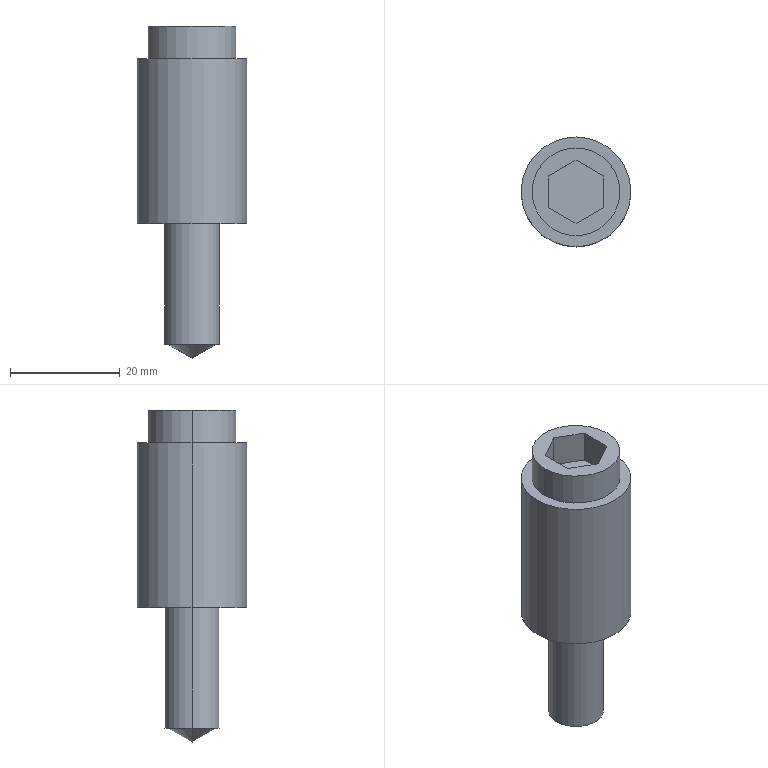Part | Creo | 1 solid | 19 faces | box 20 x 20 x 60.51 mm | volume 11893 mm3 | plane 11 | cylinder 6 | cone 2 | commonest cylinder face diameters 10 x2 16 x2 20 x2
STEP:
#1=CARTESIAN_POINT('',(-211.,254.,30.5));
#2=VERTEX_POINT('',#1);
#3=CARTESIAN_POINT('',(-195.,254.,30.5));
#4=VERTEX_POINT('',#3);
#5=CARTESIAN_POINT('',(-203.,254.,30.5));
#6=DIRECTION('',(0.,0.,1.));
#7=DIRECTION('',(-1.,0.,0.));
#8=AXIS2_PLACEMENT_3D('',#5,#6,#7);
#9=CIRCLE('',#8,8.);
#10=EDGE_CURVE('',#2,#4,#9,.T.);
#11=ORIENTED_EDGE('',*,*,#10,.F.);
#12=CARTESIAN_POINT('',(-203.,254.,30.5));
#13=DIRECTION('',(0.,0.,1.));
#14=DIRECTION('',(1.,0.,0.));
#15=AXIS2_PLACEMENT_3D('',#12,#13,#14);
#16=CIRCLE('',#15,8.);
#17=EDGE_CURVE('',#4,#2,#16,.T.);
#18=ORIENTED_EDGE('',*,*,#17,.F.);
#19=EDGE_LOOP('',(#11,#18));
#20=FACE_OUTER_BOUND('',#19,.F.);
#21=CARTESIAN_POINT('',(-198.,251.113,30.5));
#22=VERTEX_POINT('',#21);
#23=CARTESIAN_POINT('',(-203.,248.226,30.5));
#24=VERTEX_POINT('',#23);
#25=CARTESIAN_POINT('',(-198.,251.113,30.5));
#26=DIRECTION('',(-0.866,-0.5,0.));
#27=VECTOR('',#26,5.774);
#28=LINE('',#25,#27);
#29=EDGE_CURVE('',#22,#24,#28,.T.);
#30=ORIENTED_EDGE('',*,*,#29,.F.);
#31=CARTESIAN_POINT('',(-198.,256.887,30.5));
#32=VERTEX_POINT('',#31);
#33=CARTESIAN_POINT('',(-198.,251.113,30.5));
#34=DIRECTION('',(0.,1.,0.));
#35=VECTOR('',#34,5.774);
#36=LINE('',#33,#35);
#37=EDGE_CURVE('',#22,#32,#36,.T.);
#38=ORIENTED_EDGE('',*,*,#37,.T.);
#39=CARTESIAN_POINT('',(-203.,259.774,30.5));
#40=VERTEX_POINT('',#39);
#41=CARTESIAN_POINT('',(-203.,259.774,30.5));
#42=DIRECTION('',(0.866,-0.5,0.));
#43=VECTOR('',#42,5.774);
#44=LINE('',#41,#43);
#45=EDGE_CURVE('',#40,#32,#44,.T.);
#46=ORIENTED_EDGE('',*,*,#45,.F.);
#47=CARTESIAN_POINT('',(-208.,256.887,30.5));
#48=VERTEX_POINT('',#47);
#49=CARTESIAN_POINT('',(-208.,256.887,30.5));
#50=DIRECTION('',(0.866,0.5,0.));
#51=VECTOR('',#50,5.774);
#52=LINE('',#49,#51);
#53=EDGE_CURVE('',#48,#40,#52,.T.);
#54=ORIENTED_EDGE('',*,*,#53,.F.);
#55=CARTESIAN_POINT('',(-208.,251.113,30.5));
#56=VERTEX_POINT('',#55);
#57=CARTESIAN_POINT('',(-208.,256.887,30.5));
#58=DIRECTION('',(0.,-1.,0.));
#59=VECTOR('',#58,5.774);
#60=LINE('',#57,#59);
#61=EDGE_CURVE('',#48,#56,#60,.T.);
#62=ORIENTED_EDGE('',*,*,#61,.T.);
#63=CARTESIAN_POINT('',(-203.,248.226,30.5));
#64=DIRECTION('',(-0.866,0.5,0.));
#65=VECTOR('',#64,5.774);
#66=LINE('',#63,#65);
#67=EDGE_CURVE('',#24,#56,#66,.T.);
#68=ORIENTED_EDGE('',*,*,#67,.F.);
#69=EDGE_LOOP('',(#30,#38,#46,#54,#62,#68));
#70=FACE_BOUND('',#69,.F.);
#71=CARTESIAN_POINT('',(-203.,254.,30.5));
#72=DIRECTION('',(0.,0.,1.));
#73=DIRECTION('',(1.,0.,0.));
#74=AXIS2_PLACEMENT_3D('',#71,#72,#73);
#75=PLANE('',#74);
#76=ADVANCED_FACE('',(#20,#70),#75,.T.);
#77=CARTESIAN_POINT('',(-195.,254.,24.5));
#78=VERTEX_POINT('',#77);
#79=CARTESIAN_POINT('',(-211.,254.,24.5));
#80=VERTEX_POINT('',#79);
#81=CARTESIAN_POINT('',(-203.,254.,24.5));
#82=DIRECTION('',(0.,0.,-1.));
#83=DIRECTION('',(1.,0.,0.));
#84=AXIS2_PLACEMENT_3D('',#81,#82,#83);
#85=CIRCLE('',#84,8.);
#86=EDGE_CURVE('',#78,#80,#85,.T.);
#87=ORIENTED_EDGE('',*,*,#86,.T.);
#88=CARTESIAN_POINT('',(-211.,254.,24.5));
#89=DIRECTION('',(0.,0.,1.));
#90=VECTOR('',#89,6.);
#91=LINE('',#88,#90);
#92=EDGE_CURVE('',#80,#2,#91,.T.);
#93=ORIENTED_EDGE('',*,*,#92,.T.);
#94=ORIENTED_EDGE('',*,*,#10,.T.);
#95=CARTESIAN_POINT('',(-195.,254.,24.5));
#96=DIRECTION('',(0.,0.,1.));
#97=VECTOR('',#96,6.);
#98=LINE('',#95,#97);
#99=EDGE_CURVE('',#78,#4,#98,.T.);
#100=ORIENTED_EDGE('',*,*,#99,.F.);
#101=EDGE_LOOP('',(#87,#93,#94,#100));
#102=FACE_OUTER_BOUND('',#101,.F.);
#103=CARTESIAN_POINT('',(-203.,254.,-5.5));
#104=DIRECTION('',(0.,0.,1.));
#105=DIRECTION('',(1.,0.,0.));
#106=AXIS2_PLACEMENT_3D('',#103,#104,#105);
#107=CYLINDRICAL_SURFACE('',#106,8.);
#108=ADVANCED_FACE('',(#102),#107,.T.);
#109=CARTESIAN_POINT('',(-213.,254.,24.5));
#110=VERTEX_POINT('',#109);
#111=CARTESIAN_POINT('',(-193.,254.,24.5));
#112=VERTEX_POINT('',#111);
#113=CARTESIAN_POINT('',(-203.,254.,24.5));
#114=DIRECTION('',(0.,0.,1.));
#115=DIRECTION('',(-1.,0.,0.));
#116=AXIS2_PLACEMENT_3D('',#113,#114,#115);
#117=CIRCLE('',#116,10.);
#118=EDGE_CURVE('',#110,#112,#117,.T.);
#119=ORIENTED_EDGE('',*,*,#118,.F.);
#120=CARTESIAN_POINT('',(-203.,254.,24.5));
#121=DIRECTION('',(0.,0.,1.));
#122=DIRECTION('',(1.,0.,0.));
#123=AXIS2_PLACEMENT_3D('',#120,#121,#122);
#124=CIRCLE('',#123,10.);
#125=EDGE_CURVE('',#112,#110,#124,.T.);
#126=ORIENTED_EDGE('',*,*,#125,.F.);
#127=EDGE_LOOP('',(#119,#126));
#128=FACE_OUTER_BOUND('',#127,.F.);
#129=ORIENTED_EDGE('',*,*,#86,.F.);
#130=CARTESIAN_POINT('',(-203.,254.,24.5));
#131=DIRECTION('',(0.,0.,-1.));
#132=DIRECTION('',(-1.,0.,0.));
#133=AXIS2_PLACEMENT_3D('',#130,#131,#132);
#134=CIRCLE('',#133,8.);
#135=EDGE_CURVE('',#80,#78,#134,.T.);
#136=ORIENTED_EDGE('',*,*,#135,.F.);
#137=EDGE_LOOP('',(#129,#136));
#138=FACE_BOUND('',#137,.F.);
#139=CARTESIAN_POINT('',(-203.,254.,24.5));
#140=DIRECTION('',(0.,0.,1.));
#141=DIRECTION('',(1.,0.,0.));
#142=AXIS2_PLACEMENT_3D('',#139,#140,#141);
#143=PLANE('',#142);
#144=ADVANCED_FACE('',(#128,#138),#143,.T.);
#145=ORIENTED_EDGE('',*,*,#135,.T.);
#146=ORIENTED_EDGE('',*,*,#99,.T.);
#147=ORIENTED_EDGE('',*,*,#17,.T.);
#148=ORIENTED_EDGE('',*,*,#92,.F.);
#149=EDGE_LOOP('',(#145,#146,#147,#148));
#150=FACE_OUTER_BOUND('',#149,.F.);
#151=CARTESIAN_POINT('',(-203.,254.,-5.5));
#152=DIRECTION('',(0.,0.,1.));
#153=DIRECTION('',(1.,0.,0.));
#154=AXIS2_PLACEMENT_3D('',#151,#152,#153);
#155=CYLINDRICAL_SURFACE('',#154,8.);
#156=ADVANCED_FACE('',(#150),#155,.T.);
#157=ORIENTED_EDGE('',*,*,#118,.T.);
#158=CARTESIAN_POINT('',(-193.,254.,-5.5));
#159=VERTEX_POINT('',#158);
#160=CARTESIAN_POINT('',(-193.,254.,-5.5));
#161=DIRECTION('',(0.,0.,1.));
#162=VECTOR('',#161,30.);
#163=LINE('',#160,#162);
#164=EDGE_CURVE('',#159,#112,#163,.T.);
#165=ORIENTED_EDGE('',*,*,#164,.F.);
#166=CARTESIAN_POINT('',(-213.,254.,-5.5));
#167=VERTEX_POINT('',#166);
#168=CARTESIAN_POINT('',(-203.,254.,-5.5));
#169=DIRECTION('',(0.,0.,-1.));
#170=DIRECTION('',(1.,0.,0.));
#171=AXIS2_PLACEMENT_3D('',#168,#169,#170);
#172=CIRCLE('',#171,10.);
#173=EDGE_CURVE('',#159,#167,#172,.T.);
#174=ORIENTED_EDGE('',*,*,#173,.T.);
#175=CARTESIAN_POINT('',(-213.,254.,-5.5));
#176=DIRECTION('',(0.,0.,1.));
#177=VECTOR('',#176,30.);
#178=LINE('',#175,#177);
#179=EDGE_CURVE('',#167,#110,#178,.T.);
#180=ORIENTED_EDGE('',*,*,#179,.T.);
#181=EDGE_LOOP('',(#157,#165,#174,#180));
#182=FACE_OUTER_BOUND('',#181,.F.);
#183=CARTESIAN_POINT('',(-203.,254.,-5.5));
#184=DIRECTION('',(0.,0.,1.));
#185=DIRECTION('',(1.,0.,0.));
#186=AXIS2_PLACEMENT_3D('',#183,#184,#185);
#187=CYLINDRICAL_SURFACE('',#186,10.);
#188=ADVANCED_FACE('',(#182),#187,.T.);
#189=ORIENTED_EDGE('',*,*,#125,.T.);
#190=ORIENTED_EDGE('',*,*,#179,.F.);
#191=CARTESIAN_POINT('',(-203.,254.,-5.5));
#192=DIRECTION('',(0.,0.,-1.));
#193=DIRECTION('',(-1.,0.,0.));
#194=AXIS2_PLACEMENT_3D('',#191,#192,#193);
#195=CIRCLE('',#194,10.);
#196=EDGE_CURVE('',#167,#159,#195,.T.);
#197=ORIENTED_EDGE('',*,*,#196,.T.);
#198=ORIENTED_EDGE('',*,*,#164,.T.);
#199=EDGE_LOOP('',(#189,#190,#197,#198));
#200=FACE_OUTER_BOUND('',#199,.F.);
#201=CARTESIAN_POINT('',(-203.,254.,-5.5));
#202=DIRECTION('',(0.,0.,1.));
#203=DIRECTION('',(1.,0.,0.));
#204=AXIS2_PLACEMENT_3D('',#201,#202,#203);
#205=CYLINDRICAL_SURFACE('',#204,10.);
#206=ADVANCED_FACE('',(#200),#205,.T.);
#207=ORIENTED_EDGE('',*,*,#173,.F.);
#208=ORIENTED_EDGE('',*,*,#196,.F.);
#209=EDGE_LOOP('',(#207,#208));
#210=FACE_OUTER_BOUND('',#209,.F.);
#211=CARTESIAN_POINT('',(-208.,254.,-5.5));
#212=VERTEX_POINT('',#211);
#213=CARTESIAN_POINT('',(-198.,254.,-5.5));
#214=VERTEX_POINT('',#213);
#215=CARTESIAN_POINT('',(-203.,254.,-5.5));
#216=DIRECTION('',(0.,0.,1.));
#217=DIRECTION('',(-1.,0.,0.));
#218=AXIS2_PLACEMENT_3D('',#215,#216,#217);
#219=CIRCLE('',#218,5.);
#220=EDGE_CURVE('',#212,#214,#219,.T.);
#221=ORIENTED_EDGE('',*,*,#220,.F.);
#222=CARTESIAN_POINT('',(-203.,254.,-5.5));
#223=DIRECTION('',(0.,0.,1.));
#224=DIRECTION('',(1.,0.,0.));
#225=AXIS2_PLACEMENT_3D('',#222,#223,#224);
#226=CIRCLE('',#225,5.);
#227=EDGE_CURVE('',#214,#212,#226,.T.);
#228=ORIENTED_EDGE('',*,*,#227,.F.);
#229=EDGE_LOOP('',(#221,#228));
#230=FACE_BOUND('',#229,.F.);
#231=CARTESIAN_POINT('',(-203.,254.,-5.5));
#232=DIRECTION('',(0.,0.,-1.));
#233=DIRECTION('',(-1.,0.,0.));
#234=AXIS2_PLACEMENT_3D('',#231,#232,#233);
#235=PLANE('',#234);
#236=ADVANCED_FACE('',(#210,#230),#235,.T.);
#237=CARTESIAN_POINT('',(-198.,254.,-27.5));
#238=VERTEX_POINT('',#237);
#239=CARTESIAN_POINT('',(-208.,254.,-27.5));
#240=VERTEX_POINT('',#239);
#241=CARTESIAN_POINT('',(-203.,254.,-27.5));
#242=DIRECTION('',(0.,0.,-1.));
#243=DIRECTION('',(1.,0.,0.));
#244=AXIS2_PLACEMENT_3D('',#241,#242,#243);
#245=CIRCLE('',#244,5.);
#246=EDGE_CURVE('',#238,#240,#245,.T.);
#247=ORIENTED_EDGE('',*,*,#246,.T.);
#248=CARTESIAN_POINT('',(-208.,254.,-5.5));
#249=DIRECTION('',(0.,0.,-1.));
#250=VECTOR('',#249,22.);
#251=LINE('',#248,#250);
#252=EDGE_CURVE('',#212,#240,#251,.T.);
#253=ORIENTED_EDGE('',*,*,#252,.F.);
#254=ORIENTED_EDGE('',*,*,#220,.T.);
#255=CARTESIAN_POINT('',(-198.,254.,-5.5));
#256=DIRECTION('',(0.,0.,-1.));
#257=VECTOR('',#256,22.);
#258=LINE('',#255,#257);
#259=EDGE_CURVE('',#214,#238,#258,.T.);
#260=ORIENTED_EDGE('',*,*,#259,.T.);
#261=EDGE_LOOP('',(#247,#253,#254,#260));
#262=FACE_OUTER_BOUND('',#261,.F.);
#263=CARTESIAN_POINT('',(-203.,254.,-5.5));
#264=DIRECTION('',(0.,0.,-1.));
#265=DIRECTION('',(-1.,0.,0.));
#266=AXIS2_PLACEMENT_3D('',#263,#264,#265);
#267=CYLINDRICAL_SURFACE('',#266,5.);
#268=ADVANCED_FACE('',(#262),#267,.T.);
#269=ORIENTED_EDGE('',*,*,#246,.F.);
#270=CARTESIAN_POINT('',(-203.,254.,-27.5));
#271=DIRECTION('',(0.,0.,-1.));
#272=DIRECTION('',(-1.,0.,0.));
#273=AXIS2_PLACEMENT_3D('',#270,#271,#272);
#274=CIRCLE('',#273,5.);
#275=EDGE_CURVE('',#240,#238,#274,.T.);
#276=ORIENTED_EDGE('',*,*,#275,.F.);
#277=EDGE_LOOP('',(#269,#276));
#278=FACE_OUTER_BOUND('',#277,.F.);
#279=CARTESIAN_POINT('',(-207.5,254.,-27.5));
#280=VERTEX_POINT('',#279);
#281=CARTESIAN_POINT('',(-198.5,254.,-27.5));
#282=VERTEX_POINT('',#281);
#283=CARTESIAN_POINT('',(-203.,254.,-27.5));
#284=DIRECTION('',(0.,0.,1.));
#285=DIRECTION('',(-1.,0.,0.));
#286=AXIS2_PLACEMENT_3D('',#283,#284,#285);
#287=CIRCLE('',#286,4.5);
#288=EDGE_CURVE('',#280,#282,#287,.T.);
#289=ORIENTED_EDGE('',*,*,#288,.F.);
#290=CARTESIAN_POINT('',(-203.,254.,-27.5));
#291=DIRECTION('',(0.,0.,1.));
#292=DIRECTION('',(1.,0.,0.));
#293=AXIS2_PLACEMENT_3D('',#290,#291,#292);
#294=CIRCLE('',#293,4.5);
#295=EDGE_CURVE('',#282,#280,#294,.T.);
#296=ORIENTED_EDGE('',*,*,#295,.F.);
#297=EDGE_LOOP('',(#289,#296));
#298=FACE_BOUND('',#297,.F.);
#299=CARTESIAN_POINT('',(-203.,254.,-27.5));
#300=DIRECTION('',(0.,0.,-1.));
#301=DIRECTION('',(-1.,0.,0.));
#302=AXIS2_PLACEMENT_3D('',#299,#300,#301);
#303=PLANE('',#302);
#304=ADVANCED_FACE('',(#278,#298),#303,.T.);
#305=ORIENTED_EDGE('',*,*,#288,.T.);
#306=CARTESIAN_POINT('',(-203.,254.,-30.01));
#307=VERTEX_POINT('',#306);
#308=CARTESIAN_POINT('',(-203.,254.,-30.01));
#309=DIRECTION('',(0.8733,0.,0.4871));
#310=VECTOR('',#309,5.153);
#311=LINE('',#308,#310);
#312=EDGE_CURVE('',#307,#282,#311,.T.);
#313=ORIENTED_EDGE('',*,*,#312,.F.);
#314=CARTESIAN_POINT('',(-203.,254.,-30.01));
#315=DIRECTION('',(-0.8733,0.,0.4871));
#316=VECTOR('',#315,5.153);
#317=LINE('',#314,#316);
#318=EDGE_CURVE('',#307,#280,#317,.T.);
#319=ORIENTED_EDGE('',*,*,#318,.T.);
#320=EDGE_LOOP('',(#305,#313,#319));
#321=FACE_OUTER_BOUND('',#320,.F.);
#322=CARTESIAN_POINT('',(-203.,254.,-28.73));
#323=DIRECTION('',(0.,0.,1.));
#324=DIRECTION('',(1.,0.,0.));
#325=AXIS2_PLACEMENT_3D('',#322,#323,#324);
#326=CONICAL_SURFACE('',#325,2.295,60.848);
#327=ADVANCED_FACE('',(#321),#326,.T.);
#328=ORIENTED_EDGE('',*,*,#295,.T.);
#329=ORIENTED_EDGE('',*,*,#318,.F.);
#330=ORIENTED_EDGE('',*,*,#312,.T.);
#331=EDGE_LOOP('',(#328,#329,#330));
#332=FACE_OUTER_BOUND('',#331,.F.);
#333=CARTESIAN_POINT('',(-203.,254.,-28.73));
#334=DIRECTION('',(0.,0.,1.));
#335=DIRECTION('',(1.,0.,0.));
#336=AXIS2_PLACEMENT_3D('',#333,#334,#335);
#337=CONICAL_SURFACE('',#336,2.295,60.848);
#338=ADVANCED_FACE('',(#332),#337,.T.);
#339=ORIENTED_EDGE('',*,*,#275,.T.);
#340=ORIENTED_EDGE('',*,*,#259,.F.);
#341=ORIENTED_EDGE('',*,*,#227,.T.);
#342=ORIENTED_EDGE('',*,*,#252,.T.);
#343=EDGE_LOOP('',(#339,#340,#341,#342));
#344=FACE_OUTER_BOUND('',#343,.F.);
#345=CARTESIAN_POINT('',(-203.,254.,-5.5));
#346=DIRECTION('',(0.,0.,-1.));
#347=DIRECTION('',(-1.,0.,0.));
#348=AXIS2_PLACEMENT_3D('',#345,#346,#347);
#349=CYLINDRICAL_SURFACE('',#348,5.);
#350=ADVANCED_FACE('',(#344),#349,.T.);
#351=CARTESIAN_POINT('',(-203.,248.226,24.5));
#352=VERTEX_POINT('',#351);
#353=CARTESIAN_POINT('',(-198.,251.113,24.5));
#354=VERTEX_POINT('',#353);
#355=CARTESIAN_POINT('',(-203.,248.226,24.5));
#356=DIRECTION('',(0.866,0.5,0.));
#357=VECTOR('',#356,5.774);
#358=LINE('',#355,#357);
#359=EDGE_CURVE('',#352,#354,#358,.T.);
#360=ORIENTED_EDGE('',*,*,#359,.T.);
#361=CARTESIAN_POINT('',(-198.,251.113,24.5));
#362=DIRECTION('',(0.,0.,1.));
#363=VECTOR('',#362,6.);
#364=LINE('',#361,#363);
#365=EDGE_CURVE('',#354,#22,#364,.T.);
#366=ORIENTED_EDGE('',*,*,#365,.T.);
#367=ORIENTED_EDGE('',*,*,#29,.T.);
#368=CARTESIAN_POINT('',(-203.,248.226,24.5));
#369=DIRECTION('',(0.,0.,1.));
#370=VECTOR('',#369,6.);
#371=LINE('',#368,#370);
#372=EDGE_CURVE('',#352,#24,#371,.T.);
#373=ORIENTED_EDGE('',*,*,#372,.F.);
#374=EDGE_LOOP('',(#360,#366,#367,#373));
#375=FACE_OUTER_BOUND('',#374,.F.);
#376=CARTESIAN_POINT('',(-200.5,249.67,27.5));
#377=DIRECTION('',(0.5,-0.866,0.));
#378=DIRECTION('',(0.866,0.5,0.));
#379=AXIS2_PLACEMENT_3D('',#376,#377,#378);
#380=PLANE('',#379);
#381=ADVANCED_FACE('',(#375),#380,.F.);
#382=CARTESIAN_POINT('',(-198.,256.887,24.5));
#383=VERTEX_POINT('',#382);
#384=CARTESIAN_POINT('',(-198.,251.113,24.5));
#385=DIRECTION('',(0.,1.,0.));
#386=VECTOR('',#385,5.774);
#387=LINE('',#384,#386);
#388=EDGE_CURVE('',#354,#383,#387,.T.);
#389=ORIENTED_EDGE('',*,*,#388,.F.);
#390=ORIENTED_EDGE('',*,*,#359,.F.);
#391=CARTESIAN_POINT('',(-208.,251.113,24.5));
#392=VERTEX_POINT('',#391);
#393=CARTESIAN_POINT('',(-208.,251.113,24.5));
#394=DIRECTION('',(0.866,-0.5,0.));
#395=VECTOR('',#394,5.774);
#396=LINE('',#393,#395);
#397=EDGE_CURVE('',#392,#352,#396,.T.);
#398=ORIENTED_EDGE('',*,*,#397,.F.);
#399=CARTESIAN_POINT('',(-208.,256.887,24.5));
#400=VERTEX_POINT('',#399);
#401=CARTESIAN_POINT('',(-208.,256.887,24.5));
#402=DIRECTION('',(0.,-1.,0.));
#403=VECTOR('',#402,5.774);
#404=LINE('',#401,#403);
#405=EDGE_CURVE('',#400,#392,#404,.T.);
#406=ORIENTED_EDGE('',*,*,#405,.F.);
#407=CARTESIAN_POINT('',(-203.,259.774,24.5));
#408=VERTEX_POINT('',#407);
#409=CARTESIAN_POINT('',(-203.,259.774,24.5));
#410=DIRECTION('',(-0.866,-0.5,0.));
#411=VECTOR('',#410,5.774);
#412=LINE('',#409,#411);
#413=EDGE_CURVE('',#408,#400,#412,.T.);
#414=ORIENTED_EDGE('',*,*,#413,.F.);
#415=CARTESIAN_POINT('',(-198.,256.887,24.5));
#416=DIRECTION('',(-0.866,0.5,0.));
#417=VECTOR('',#416,5.774);
#418=LINE('',#415,#417);
#419=EDGE_CURVE('',#383,#408,#418,.T.);
#420=ORIENTED_EDGE('',*,*,#419,.F.);
#421=EDGE_LOOP('',(#389,#390,#398,#406,#414,#420));
#422=FACE_OUTER_BOUND('',#421,.F.);
#423=CARTESIAN_POINT('',(-203.,254.,24.5));
#424=DIRECTION('',(0.,0.,-1.));
#425=DIRECTION('',(-1.,0.,0.));
#426=AXIS2_PLACEMENT_3D('',#423,#424,#425);
#427=PLANE('',#426);
#428=ADVANCED_FACE('',(#422),#427,.F.);
#429=ORIENTED_EDGE('',*,*,#388,.T.);
#430=CARTESIAN_POINT('',(-198.,256.887,24.5));
#431=DIRECTION('',(0.,0.,1.));
#432=VECTOR('',#431,6.);
#433=LINE('',#430,#432);
#434=EDGE_CURVE('',#383,#32,#433,.T.);
#435=ORIENTED_EDGE('',*,*,#434,.T.);
#436=ORIENTED_EDGE('',*,*,#37,.F.);
#437=ORIENTED_EDGE('',*,*,#365,.F.);
#438=EDGE_LOOP('',(#429,#435,#436,#437));
#439=FACE_OUTER_BOUND('',#438,.F.);
#440=CARTESIAN_POINT('',(-198.,254.,27.5));
#441=DIRECTION('',(1.,0.,0.));
#442=DIRECTION('',(0.,0.,-1.));
#443=AXIS2_PLACEMENT_3D('',#440,#441,#442);
#444=PLANE('',#443);
#445=ADVANCED_FACE('',(#439),#444,.F.);
#446=ORIENTED_EDGE('',*,*,#419,.T.);
#447=CARTESIAN_POINT('',(-203.,259.774,24.5));
#448=DIRECTION('',(0.,0.,1.));
#449=VECTOR('',#448,6.);
#450=LINE('',#447,#449);
#451=EDGE_CURVE('',#408,#40,#450,.T.);
#452=ORIENTED_EDGE('',*,*,#451,.T.);
#453=ORIENTED_EDGE('',*,*,#45,.T.);
#454=ORIENTED_EDGE('',*,*,#434,.F.);
#455=EDGE_LOOP('',(#446,#452,#453,#454));
#456=FACE_OUTER_BOUND('',#455,.F.);
#457=CARTESIAN_POINT('',(-200.5,258.33,27.5));
#458=DIRECTION('',(0.5,0.866,0.));
#459=DIRECTION('',(-0.866,0.5,0.));
#460=AXIS2_PLACEMENT_3D('',#457,#458,#459);
#461=PLANE('',#460);
#462=ADVANCED_FACE('',(#456),#461,.F.);
#463=ORIENTED_EDGE('',*,*,#413,.T.);
#464=CARTESIAN_POINT('',(-208.,256.887,24.5));
#465=DIRECTION('',(0.,0.,1.));
#466=VECTOR('',#465,6.);
#467=LINE('',#464,#466);
#468=EDGE_CURVE('',#400,#48,#467,.T.);
#469=ORIENTED_EDGE('',*,*,#468,.T.);
#470=ORIENTED_EDGE('',*,*,#53,.T.);
#471=ORIENTED_EDGE('',*,*,#451,.F.);
#472=EDGE_LOOP('',(#463,#469,#470,#471));
#473=FACE_OUTER_BOUND('',#472,.F.);
#474=CARTESIAN_POINT('',(-205.5,258.33,27.5));
#475=DIRECTION('',(-0.5,0.866,0.));
#476=DIRECTION('',(-0.866,-0.5,0.));
#477=AXIS2_PLACEMENT_3D('',#474,#475,#476);
#478=PLANE('',#477);
#479=ADVANCED_FACE('',(#473),#478,.F.);
#480=ORIENTED_EDGE('',*,*,#405,.T.);
#481=CARTESIAN_POINT('',(-208.,251.113,24.5));
#482=DIRECTION('',(0.,0.,1.));
#483=VECTOR('',#482,6.);
#484=LINE('',#481,#483);
#485=EDGE_CURVE('',#392,#56,#484,.T.);
#486=ORIENTED_EDGE('',*,*,#485,.T.);
#487=ORIENTED_EDGE('',*,*,#61,.F.);
#488=ORIENTED_EDGE('',*,*,#468,.F.);
#489=EDGE_LOOP('',(#480,#486,#487,#488));
#490=FACE_OUTER_BOUND('',#489,.F.);
#491=CARTESIAN_POINT('',(-208.,254.,27.5));
#492=DIRECTION('',(-1.,0.,0.));
#493=DIRECTION('',(0.,0.,1.));
#494=AXIS2_PLACEMENT_3D('',#491,#492,#493);
#495=PLANE('',#494);
#496=ADVANCED_FACE('',(#490),#495,.F.);
#497=ORIENTED_EDGE('',*,*,#397,.T.);
#498=ORIENTED_EDGE('',*,*,#372,.T.);
#499=ORIENTED_EDGE('',*,*,#67,.T.);
#500=ORIENTED_EDGE('',*,*,#485,.F.);
#501=EDGE_LOOP('',(#497,#498,#499,#500));
#502=FACE_OUTER_BOUND('',#501,.F.);
#503=CARTESIAN_POINT('',(-205.5,249.67,27.5));
#504=DIRECTION('',(-0.5,-0.866,0.));
#505=DIRECTION('',(0.866,-0.5,0.));
#506=AXIS2_PLACEMENT_3D('',#503,#504,#505);
#507=PLANE('',#506);
#508=ADVANCED_FACE('',(#502),#507,.F.);
#509=CLOSED_SHELL('',(#76,#108,#144,#156,#188,#206,#236,#268,#304,#327,#338,#350,#381,#428,#445,#462,#479,#496,#508));
#510=MANIFOLD_SOLID_BREP('',#509);
#511=(LENGTH_UNIT()NAMED_UNIT(*)SI_UNIT(.MILLI.,.METRE.));
#512=UNCERTAINTY_MEASURE_WITH_UNIT(LENGTH_MEASURE(0.00668),#511,'','');
#513=(NAMED_UNIT(*)PLANE_ANGLE_UNIT()SI_UNIT($,.RADIAN.));
#514=PLANE_ANGLE_MEASURE_WITH_UNIT(PLANE_ANGLE_MEASURE(0.01745),#513);
#515=(CONVERSION_BASED_UNIT('DEGREE',#514)NAMED_UNIT(*)PLANE_ANGLE_UNIT());
#516=(NAMED_UNIT(*)SI_UNIT($,.STERADIAN.)SOLID_ANGLE_UNIT());
#517=(GEOMETRIC_REPRESENTATION_CONTEXT(3)GLOBAL_UNCERTAINTY_ASSIGNED_CONTEXT((#512))GLOBAL_UNIT_ASSIGNED_CONTEXT((#511,#515,#516))REPRESENTATION_CONTEXT('',''));
#518=ADVANCED_BREP_SHAPE_REPRESENTATION('',(#510),#517);